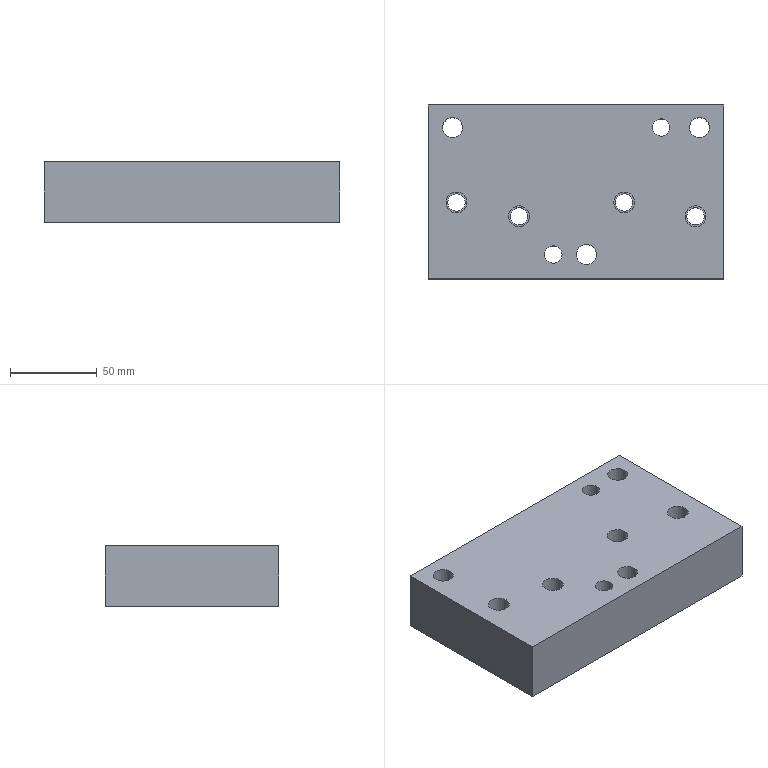Part | NX | features solid 2 | 1 solid | 45 faces | box 170 x 100 x 35 mm | volume 548006 mm3 | cylinder 24 | plane 13 | cone 8 | commonest cylinder face diameters 8.506 x8 10 x6 12 x4 11.509 x3 18.007 x3
STEP:
#1=CARTESIAN_POINT('',(1400.579,138.904,53.));
#2=VERTEX_POINT('',#1);
#3=CARTESIAN_POINT('',(1405.579,138.904,53.));
#4=DIRECTION('',(0.,0.,-1.));
#5=DIRECTION('',(-1.,0.,0.));
#6=AXIS2_PLACEMENT_3D('',#3,#4,#5);
#7=CIRCLE('',#6,5.);
#8=EDGE_CURVE('',#2,#2,#7,.T.);
#9=ORIENTED_EDGE('',*,*,#8,.F.);
#10=EDGE_LOOP('',(#9));
#11=FACE_BOUND('',#10,.T.);
#12=CARTESIAN_POINT('',(1359.579,146.904,53.));
#13=VERTEX_POINT('',#12);
#14=CARTESIAN_POINT('',(1364.579,146.904,53.));
#15=DIRECTION('',(0.,0.,-1.));
#16=DIRECTION('',(-1.,0.,0.));
#17=AXIS2_PLACEMENT_3D('',#14,#15,#16);
#18=CIRCLE('',#17,5.);
#19=EDGE_CURVE('',#13,#13,#18,.T.);
#20=ORIENTED_EDGE('',*,*,#19,.F.);
#21=EDGE_LOOP('',(#20));
#22=FACE_BOUND('',#21,.T.);
#23=CARTESIAN_POINT('',(1299.079,138.904,53.));
#24=VERTEX_POINT('',#23);
#25=CARTESIAN_POINT('',(1304.079,138.904,53.));
#26=DIRECTION('',(0.,0.,-1.));
#27=DIRECTION('',(-1.,0.,0.));
#28=AXIS2_PLACEMENT_3D('',#25,#26,#27);
#29=CIRCLE('',#28,5.);
#30=EDGE_CURVE('',#24,#24,#29,.T.);
#31=ORIENTED_EDGE('',*,*,#30,.F.);
#32=EDGE_LOOP('',(#31));
#33=FACE_BOUND('',#32,.T.);
#34=CARTESIAN_POINT('',(1263.079,146.904,53.));
#35=VERTEX_POINT('',#34);
#36=CARTESIAN_POINT('',(1268.079,146.904,53.));
#37=DIRECTION('',(0.,0.,-1.));
#38=DIRECTION('',(-1.,0.,0.));
#39=AXIS2_PLACEMENT_3D('',#36,#37,#38);
#40=CIRCLE('',#39,5.);
#41=EDGE_CURVE('',#35,#35,#40,.T.);
#42=ORIENTED_EDGE('',*,*,#41,.F.);
#43=EDGE_LOOP('',(#42));
#44=FACE_BOUND('',#43,.T.);
#45=CARTESIAN_POINT('',(1360.326,122.904,53.));
#46=VERTEX_POINT('',#45);
#47=CARTESIAN_POINT('',(1364.579,122.904,53.));
#48=DIRECTION('',(0.,0.,-1.));
#49=DIRECTION('',(-1.,0.,0.));
#50=AXIS2_PLACEMENT_3D('',#47,#48,#49);
#51=CIRCLE('',#50,4.253);
#52=EDGE_CURVE('',#46,#46,#51,.T.);
#53=ORIENTED_EDGE('',*,*,#52,.F.);
#54=EDGE_LOOP('',(#53));
#55=FACE_BOUND('',#54,.T.);
#56=CARTESIAN_POINT('',(1263.826,122.904,53.));
#57=VERTEX_POINT('',#56);
#58=CARTESIAN_POINT('',(1268.079,122.904,53.));
#59=DIRECTION('',(0.,0.,-1.));
#60=DIRECTION('',(-1.,0.,0.));
#61=AXIS2_PLACEMENT_3D('',#58,#59,#60);
#62=CIRCLE('',#61,4.253);
#63=EDGE_CURVE('',#57,#57,#62,.T.);
#64=ORIENTED_EDGE('',*,*,#63,.F.);
#65=EDGE_LOOP('',(#64));
#66=FACE_BOUND('',#65,.T.);
#67=CARTESIAN_POINT('',(1299.826,118.904,53.));
#68=VERTEX_POINT('',#67);
#69=CARTESIAN_POINT('',(1304.079,118.904,53.));
#70=DIRECTION('',(0.,0.,-1.));
#71=DIRECTION('',(-1.,0.,0.));
#72=AXIS2_PLACEMENT_3D('',#69,#70,#71);
#73=CIRCLE('',#72,4.253);
#74=EDGE_CURVE('',#68,#68,#73,.T.);
#75=ORIENTED_EDGE('',*,*,#74,.F.);
#76=EDGE_LOOP('',(#75));
#77=FACE_BOUND('',#76,.T.);
#78=CARTESIAN_POINT('',(1299.826,164.904,53.));
#79=VERTEX_POINT('',#78);
#80=CARTESIAN_POINT('',(1304.079,164.904,53.));
#81=DIRECTION('',(0.,0.,-1.));
#82=DIRECTION('',(-1.,0.,0.));
#83=AXIS2_PLACEMENT_3D('',#80,#81,#82);
#84=CIRCLE('',#83,4.253);
#85=EDGE_CURVE('',#79,#79,#84,.T.);
#86=ORIENTED_EDGE('',*,*,#85,.F.);
#87=EDGE_LOOP('',(#86));
#88=FACE_BOUND('',#87,.T.);
#89=CARTESIAN_POINT('',(1401.326,118.904,53.));
#90=VERTEX_POINT('',#89);
#91=CARTESIAN_POINT('',(1405.579,118.904,53.));
#92=DIRECTION('',(0.,0.,-1.));
#93=DIRECTION('',(-1.,0.,0.));
#94=AXIS2_PLACEMENT_3D('',#91,#92,#93);
#95=CIRCLE('',#94,4.253);
#96=EDGE_CURVE('',#90,#90,#95,.T.);
#97=ORIENTED_EDGE('',*,*,#96,.F.);
#98=EDGE_LOOP('',(#97));
#99=FACE_BOUND('',#98,.T.);
#100=CARTESIAN_POINT('',(1401.326,164.904,53.));
#101=VERTEX_POINT('',#100);
#102=CARTESIAN_POINT('',(1405.579,164.904,53.));
#103=DIRECTION('',(0.,0.,-1.));
#104=DIRECTION('',(-1.,0.,0.));
#105=AXIS2_PLACEMENT_3D('',#102,#103,#104);
#106=CIRCLE('',#105,4.253);
#107=EDGE_CURVE('',#101,#101,#106,.T.);
#108=ORIENTED_EDGE('',*,*,#107,.F.);
#109=EDGE_LOOP('',(#108));
#110=FACE_BOUND('',#109,.T.);
#111=CARTESIAN_POINT('',(1360.326,164.904,53.));
#112=VERTEX_POINT('',#111);
#113=CARTESIAN_POINT('',(1364.579,164.904,53.));
#114=DIRECTION('',(0.,0.,-1.));
#115=DIRECTION('',(-1.,0.,0.));
#116=AXIS2_PLACEMENT_3D('',#113,#114,#115);
#117=CIRCLE('',#116,4.253);
#118=EDGE_CURVE('',#112,#112,#117,.T.);
#119=ORIENTED_EDGE('',*,*,#118,.F.);
#120=EDGE_LOOP('',(#119));
#121=FACE_BOUND('',#120,.T.);
#122=CARTESIAN_POINT('',(1263.826,164.904,53.));
#123=VERTEX_POINT('',#122);
#124=CARTESIAN_POINT('',(1268.079,164.904,53.));
#125=DIRECTION('',(0.,0.,-1.));
#126=DIRECTION('',(-1.,0.,0.));
#127=AXIS2_PLACEMENT_3D('',#124,#125,#126);
#128=CIRCLE('',#127,4.253);
#129=EDGE_CURVE('',#123,#123,#128,.T.);
#130=ORIENTED_EDGE('',*,*,#129,.F.);
#131=EDGE_LOOP('',(#130));
#132=FACE_BOUND('',#131,.T.);
#133=CARTESIAN_POINT('',(1398.825,189.904,53.));
#134=VERTEX_POINT('',#133);
#135=CARTESIAN_POINT('',(1407.829,189.904,53.));
#136=DIRECTION('',(0.,0.,-1.));
#137=DIRECTION('',(-1.,0.,0.));
#138=AXIS2_PLACEMENT_3D('',#135,#136,#137);
#139=CIRCLE('',#138,9.004);
#140=EDGE_CURVE('',#134,#134,#139,.T.);
#141=ORIENTED_EDGE('',*,*,#140,.F.);
#142=EDGE_LOOP('',(#141));
#143=FACE_BOUND('',#142,.T.);
#144=CARTESIAN_POINT('',(1421.829,202.904,53.));
#145=VERTEX_POINT('',#144);
#146=CARTESIAN_POINT('',(1421.829,102.904,53.));
#147=VERTEX_POINT('',#146);
#148=CARTESIAN_POINT('',(1421.829,141.904,53.));
#149=DIRECTION('',(0.,-1.,0.));
#150=VECTOR('',#149,1000.);
#151=LINE('',#148,#150);
#152=EDGE_CURVE('',#145,#147,#151,.T.);
#153=ORIENTED_EDGE('',*,*,#152,.T.);
#154=CARTESIAN_POINT('',(1251.829,102.904,53.));
#155=VERTEX_POINT('',#154);
#156=CARTESIAN_POINT('',(1336.829,102.904,53.));
#157=DIRECTION('',(-1.,0.,0.));
#158=VECTOR('',#157,1000.);
#159=LINE('',#156,#158);
#160=EDGE_CURVE('',#147,#155,#159,.T.);
#161=ORIENTED_EDGE('',*,*,#160,.T.);
#162=CARTESIAN_POINT('',(1251.829,202.904,53.));
#163=VERTEX_POINT('',#162);
#164=CARTESIAN_POINT('',(1251.829,141.904,53.));
#165=DIRECTION('',(0.,1.,0.));
#166=VECTOR('',#165,1000.);
#167=LINE('',#164,#166);
#168=EDGE_CURVE('',#155,#163,#167,.T.);
#169=ORIENTED_EDGE('',*,*,#168,.T.);
#170=CARTESIAN_POINT('',(1336.829,202.904,53.));
#171=DIRECTION('',(1.,0.,0.));
#172=VECTOR('',#171,1000.);
#173=LINE('',#170,#172);
#174=EDGE_CURVE('',#163,#145,#173,.T.);
#175=ORIENTED_EDGE('',*,*,#174,.T.);
#176=EDGE_LOOP('',(#153,#161,#169,#175));
#177=FACE_BOUND('',#176,.T.);
#178=CARTESIAN_POINT('',(1380.829,189.904,53.));
#179=VERTEX_POINT('',#178);
#180=CARTESIAN_POINT('',(1385.829,189.904,53.));
#181=DIRECTION('',(0.,0.,-1.));
#182=DIRECTION('',(-1.,0.,0.));
#183=AXIS2_PLACEMENT_3D('',#180,#181,#182);
#184=CIRCLE('',#183,5.);
#185=EDGE_CURVE('',#179,#179,#184,.F.);
#186=ORIENTED_EDGE('',*,*,#185,.T.);
#187=EDGE_LOOP('',(#186));
#188=FACE_BOUND('',#187,.T.);
#189=CARTESIAN_POINT('',(1318.829,116.904,53.));
#190=VERTEX_POINT('',#189);
#191=CARTESIAN_POINT('',(1323.829,116.904,53.));
#192=DIRECTION('',(0.,0.,-1.));
#193=DIRECTION('',(-1.,0.,0.));
#194=AXIS2_PLACEMENT_3D('',#191,#192,#193);
#195=CIRCLE('',#194,5.);
#196=EDGE_CURVE('',#190,#190,#195,.F.);
#197=ORIENTED_EDGE('',*,*,#196,.T.);
#198=EDGE_LOOP('',(#197));
#199=FACE_BOUND('',#198,.T.);
#200=CARTESIAN_POINT('',(1333.825,116.904,53.));
#201=VERTEX_POINT('',#200);
#202=CARTESIAN_POINT('',(1342.829,116.904,53.));
#203=DIRECTION('',(0.,0.,-1.));
#204=DIRECTION('',(-1.,0.,0.));
#205=AXIS2_PLACEMENT_3D('',#202,#203,#204);
#206=CIRCLE('',#205,9.004);
#207=EDGE_CURVE('',#201,#201,#206,.T.);
#208=ORIENTED_EDGE('',*,*,#207,.F.);
#209=EDGE_LOOP('',(#208));
#210=FACE_BOUND('',#209,.T.);
#211=CARTESIAN_POINT('',(1256.825,189.904,53.));
#212=VERTEX_POINT('',#211);
#213=CARTESIAN_POINT('',(1265.829,189.904,53.));
#214=DIRECTION('',(0.,0.,-1.));
#215=DIRECTION('',(-1.,0.,0.));
#216=AXIS2_PLACEMENT_3D('',#213,#214,#215);
#217=CIRCLE('',#216,9.004);
#218=EDGE_CURVE('',#212,#212,#217,.T.);
#219=ORIENTED_EDGE('',*,*,#218,.F.);
#220=EDGE_LOOP('',(#219));
#221=FACE_BOUND('',#220,.T.);
#222=CARTESIAN_POINT('',(1336.829,141.904,53.));
#223=DIRECTION('',(0.,0.,-1.));
#224=DIRECTION('',(-1.,0.,0.));
#225=AXIS2_PLACEMENT_3D('',#222,#223,#224);
#226=PLANE('',#225);
#227=ADVANCED_FACE('',(#11,#22,#33,#44,#55,#66,#77,#88,#99,#110,#121,#132,#143,#177,#188,#199,#210,#221),#226,.T.);
#228=CARTESIAN_POINT('',(1421.829,202.904,88.));
#229=VERTEX_POINT('',#228);
#230=CARTESIAN_POINT('',(1251.829,202.904,88.));
#231=VERTEX_POINT('',#230);
#232=CARTESIAN_POINT('',(1336.829,202.904,88.));
#233=DIRECTION('',(-1.,0.,0.));
#234=VECTOR('',#233,1000.);
#235=LINE('',#232,#234);
#236=EDGE_CURVE('',#229,#231,#235,.T.);
#237=ORIENTED_EDGE('',*,*,#236,.F.);
#238=CARTESIAN_POINT('',(1421.829,202.904,50.));
#239=DIRECTION('',(0.,0.,1.));
#240=VECTOR('',#239,1000.);
#241=LINE('',#238,#240);
#242=EDGE_CURVE('',#145,#229,#241,.T.);
#243=ORIENTED_EDGE('',*,*,#242,.F.);
#244=ORIENTED_EDGE('',*,*,#174,.F.);
#245=CARTESIAN_POINT('',(1251.829,202.904,50.));
#246=DIRECTION('',(0.,0.,1.));
#247=VECTOR('',#246,1000.);
#248=LINE('',#245,#247);
#249=EDGE_CURVE('',#163,#231,#248,.T.);
#250=ORIENTED_EDGE('',*,*,#249,.T.);
#251=EDGE_LOOP('',(#237,#243,#244,#250));
#252=FACE_BOUND('',#251,.T.);
#253=CARTESIAN_POINT('',(1336.829,202.904,50.));
#254=DIRECTION('',(0.,1.,0.));
#255=DIRECTION('',(0.,0.,-1.));
#256=AXIS2_PLACEMENT_3D('',#253,#254,#255);
#257=PLANE('',#256);
#258=ADVANCED_FACE('',(#252),#257,.T.);
#259=CARTESIAN_POINT('',(1251.829,102.904,88.));
#260=VERTEX_POINT('',#259);
#261=CARTESIAN_POINT('',(1251.829,141.904,88.));
#262=DIRECTION('',(0.,-1.,0.));
#263=VECTOR('',#262,1000.);
#264=LINE('',#261,#263);
#265=EDGE_CURVE('',#231,#260,#264,.T.);
#266=ORIENTED_EDGE('',*,*,#265,.F.);
#267=ORIENTED_EDGE('',*,*,#249,.F.);
#268=ORIENTED_EDGE('',*,*,#168,.F.);
#269=CARTESIAN_POINT('',(1251.829,102.904,50.));
#270=DIRECTION('',(0.,0.,1.));
#271=VECTOR('',#270,1000.);
#272=LINE('',#269,#271);
#273=EDGE_CURVE('',#155,#260,#272,.T.);
#274=ORIENTED_EDGE('',*,*,#273,.T.);
#275=EDGE_LOOP('',(#266,#267,#268,#274));
#276=FACE_BOUND('',#275,.T.);
#277=CARTESIAN_POINT('',(1251.829,141.904,50.));
#278=DIRECTION('',(-1.,0.,0.));
#279=DIRECTION('',(0.,0.,1.));
#280=AXIS2_PLACEMENT_3D('',#277,#278,#279);
#281=PLANE('',#280);
#282=ADVANCED_FACE('',(#276),#281,.T.);
#283=CARTESIAN_POINT('',(1421.829,102.904,88.));
#284=VERTEX_POINT('',#283);
#285=CARTESIAN_POINT('',(1336.829,102.904,88.));
#286=DIRECTION('',(-1.,0.,0.));
#287=VECTOR('',#286,1000.);
#288=LINE('',#285,#287);
#289=EDGE_CURVE('',#284,#260,#288,.T.);
#290=ORIENTED_EDGE('',*,*,#289,.T.);
#291=ORIENTED_EDGE('',*,*,#273,.F.);
#292=ORIENTED_EDGE('',*,*,#160,.F.);
#293=CARTESIAN_POINT('',(1421.829,102.904,50.));
#294=DIRECTION('',(0.,0.,1.));
#295=VECTOR('',#294,1000.);
#296=LINE('',#293,#295);
#297=EDGE_CURVE('',#147,#284,#296,.T.);
#298=ORIENTED_EDGE('',*,*,#297,.T.);
#299=EDGE_LOOP('',(#290,#291,#292,#298));
#300=FACE_BOUND('',#299,.T.);
#301=CARTESIAN_POINT('',(1336.829,102.904,50.));
#302=DIRECTION('',(0.,-1.,0.));
#303=DIRECTION('',(0.,0.,1.));
#304=AXIS2_PLACEMENT_3D('',#301,#302,#303);
#305=PLANE('',#304);
#306=ADVANCED_FACE('',(#300),#305,.T.);
#307=CARTESIAN_POINT('',(1421.829,141.904,88.));
#308=DIRECTION('',(0.,-1.,0.));
#309=VECTOR('',#308,1000.);
#310=LINE('',#307,#309);
#311=EDGE_CURVE('',#229,#284,#310,.T.);
#312=ORIENTED_EDGE('',*,*,#311,.T.);
#313=ORIENTED_EDGE('',*,*,#297,.F.);
#314=ORIENTED_EDGE('',*,*,#152,.F.);
#315=ORIENTED_EDGE('',*,*,#242,.T.);
#316=EDGE_LOOP('',(#312,#313,#314,#315));
#317=FACE_BOUND('',#316,.T.);
#318=CARTESIAN_POINT('',(1421.829,141.904,50.));
#319=DIRECTION('',(1.,0.,0.));
#320=DIRECTION('',(0.,0.,-1.));
#321=AXIS2_PLACEMENT_3D('',#318,#319,#320);
#322=PLANE('',#321);
#323=ADVANCED_FACE('',(#317),#322,.T.);
#324=CARTESIAN_POINT('',(1399.579,138.904,88.));
#325=VERTEX_POINT('',#324);
#326=CARTESIAN_POINT('',(1405.579,138.904,88.));
#327=DIRECTION('',(0.,0.,-1.));
#328=DIRECTION('',(-1.,0.,0.));
#329=AXIS2_PLACEMENT_3D('',#326,#327,#328);
#330=CIRCLE('',#329,6.);
#331=EDGE_CURVE('',#325,#325,#330,.T.);
#332=ORIENTED_EDGE('',*,*,#331,.T.);
#333=EDGE_LOOP('',(#332));
#334=FACE_BOUND('',#333,.T.);
#335=CARTESIAN_POINT('',(1358.579,146.904,88.));
#336=VERTEX_POINT('',#335);
#337=CARTESIAN_POINT('',(1364.579,146.904,88.));
#338=DIRECTION('',(0.,0.,-1.));
#339=DIRECTION('',(-1.,0.,0.));
#340=AXIS2_PLACEMENT_3D('',#337,#338,#339);
#341=CIRCLE('',#340,6.);
#342=EDGE_CURVE('',#336,#336,#341,.T.);
#343=ORIENTED_EDGE('',*,*,#342,.T.);
#344=EDGE_LOOP('',(#343));
#345=FACE_BOUND('',#344,.T.);
#346=CARTESIAN_POINT('',(1298.079,138.904,88.));
#347=VERTEX_POINT('',#346);
#348=CARTESIAN_POINT('',(1304.079,138.904,88.));
#349=DIRECTION('',(0.,0.,-1.));
#350=DIRECTION('',(-1.,0.,0.));
#351=AXIS2_PLACEMENT_3D('',#348,#349,#350);
#352=CIRCLE('',#351,6.);
#353=EDGE_CURVE('',#347,#347,#352,.T.);
#354=ORIENTED_EDGE('',*,*,#353,.T.);
#355=EDGE_LOOP('',(#354));
#356=FACE_BOUND('',#355,.T.);
#357=CARTESIAN_POINT('',(1262.079,146.904,88.));
#358=VERTEX_POINT('',#357);
#359=CARTESIAN_POINT('',(1268.079,146.904,88.));
#360=DIRECTION('',(0.,0.,-1.));
#361=DIRECTION('',(-1.,0.,0.));
#362=AXIS2_PLACEMENT_3D('',#359,#360,#361);
#363=CIRCLE('',#362,6.);
#364=EDGE_CURVE('',#358,#358,#363,.T.);
#365=ORIENTED_EDGE('',*,*,#364,.T.);
#366=EDGE_LOOP('',(#365));
#367=FACE_BOUND('',#366,.T.);
#368=CARTESIAN_POINT('',(1260.074,189.904,88.));
#369=VERTEX_POINT('',#368);
#370=CARTESIAN_POINT('',(1265.829,189.904,88.));
#371=DIRECTION('',(0.,0.,1.));
#372=DIRECTION('',(-1.,0.,0.));
#373=AXIS2_PLACEMENT_3D('',#370,#371,#372);
#374=CIRCLE('',#373,5.755);
#375=EDGE_CURVE('',#369,#369,#374,.T.);
#376=ORIENTED_EDGE('',*,*,#375,.F.);
#377=EDGE_LOOP('',(#376));
#378=FACE_BOUND('',#377,.T.);
#379=CARTESIAN_POINT('',(1318.829,116.904,88.));
#380=VERTEX_POINT('',#379);
#381=CARTESIAN_POINT('',(1323.829,116.904,88.));
#382=DIRECTION('',(0.,0.,1.));
#383=DIRECTION('',(-1.,0.,0.));
#384=AXIS2_PLACEMENT_3D('',#381,#382,#383);
#385=CIRCLE('',#384,5.);
#386=EDGE_CURVE('',#380,#380,#385,.T.);
#387=ORIENTED_EDGE('',*,*,#386,.F.);
#388=EDGE_LOOP('',(#387));
#389=FACE_BOUND('',#388,.T.);
#390=CARTESIAN_POINT('',(1380.829,189.904,88.));
#391=VERTEX_POINT('',#390);
#392=CARTESIAN_POINT('',(1385.829,189.904,88.));
#393=DIRECTION('',(0.,0.,1.));
#394=DIRECTION('',(-1.,0.,0.));
#395=AXIS2_PLACEMENT_3D('',#392,#393,#394);
#396=CIRCLE('',#395,5.);
#397=EDGE_CURVE('',#391,#391,#396,.T.);
#398=ORIENTED_EDGE('',*,*,#397,.F.);
#399=EDGE_LOOP('',(#398));
#400=FACE_BOUND('',#399,.T.);
#401=CARTESIAN_POINT('',(1402.074,189.904,88.));
#402=VERTEX_POINT('',#401);
#403=CARTESIAN_POINT('',(1407.829,189.904,88.));
#404=DIRECTION('',(0.,0.,1.));
#405=DIRECTION('',(-1.,0.,0.));
#406=AXIS2_PLACEMENT_3D('',#403,#404,#405);
#407=CIRCLE('',#406,5.755);
#408=EDGE_CURVE('',#402,#402,#407,.T.);
#409=ORIENTED_EDGE('',*,*,#408,.F.);
#410=EDGE_LOOP('',(#409));
#411=FACE_BOUND('',#410,.T.);
#412=CARTESIAN_POINT('',(1337.074,116.904,88.));
#413=VERTEX_POINT('',#412);
#414=CARTESIAN_POINT('',(1342.829,116.904,88.));
#415=DIRECTION('',(0.,0.,1.));
#416=DIRECTION('',(-1.,0.,0.));
#417=AXIS2_PLACEMENT_3D('',#414,#415,#416);
#418=CIRCLE('',#417,5.755);
#419=EDGE_CURVE('',#413,#413,#418,.T.);
#420=ORIENTED_EDGE('',*,*,#419,.F.);
#421=EDGE_LOOP('',(#420));
#422=FACE_BOUND('',#421,.T.);
#423=ORIENTED_EDGE('',*,*,#236,.T.);
#424=ORIENTED_EDGE('',*,*,#265,.T.);
#425=ORIENTED_EDGE('',*,*,#289,.F.);
#426=ORIENTED_EDGE('',*,*,#311,.F.);
#427=EDGE_LOOP('',(#423,#424,#425,#426));
#428=FACE_BOUND('',#427,.T.);
#429=CARTESIAN_POINT('',(1336.829,141.904,88.));
#430=DIRECTION('',(0.,0.,-1.));
#431=DIRECTION('',(-1.,0.,0.));
#432=AXIS2_PLACEMENT_3D('',#429,#430,#431);
#433=PLANE('',#432);
#434=ADVANCED_FACE('',(#334,#345,#356,#367,#378,#389,#400,#411,#422,#428),#433,.F.);
#435=CARTESIAN_POINT('',(1348.583,116.904,63.));
#436=VERTEX_POINT('',#435);
#437=CARTESIAN_POINT('',(1342.829,116.904,63.));
#438=DIRECTION('',(0.,0.,-1.));
#439=DIRECTION('',(1.,0.,0.));
#440=AXIS2_PLACEMENT_3D('',#437,#438,#439);
#441=CIRCLE('',#440,5.755);
#442=EDGE_CURVE('',#436,#436,#441,.T.);
#443=ORIENTED_EDGE('',*,*,#442,.T.);
#444=EDGE_LOOP('',(#443));
#445=FACE_BOUND('',#444,.T.);
#446=ORIENTED_EDGE('',*,*,#419,.T.);
#447=EDGE_LOOP('',(#446));
#448=FACE_BOUND('',#447,.T.);
#449=CARTESIAN_POINT('',(1342.829,116.904,45.));
#450=DIRECTION('',(0.,0.,1.));
#451=DIRECTION('',(1.,0.,0.));
#452=AXIS2_PLACEMENT_3D('',#449,#450,#451);
#453=CYLINDRICAL_SURFACE('',#452,5.755);
#454=ADVANCED_FACE('',(#445,#448),#453,.F.);
#455=ORIENTED_EDGE('',*,*,#442,.F.);
#456=EDGE_LOOP('',(#455));
#457=FACE_BOUND('',#456,.T.);
#458=CARTESIAN_POINT('',(1351.832,116.904,63.));
#459=VERTEX_POINT('',#458);
#460=CARTESIAN_POINT('',(1342.829,116.904,63.));
#461=DIRECTION('',(0.,0.,1.));
#462=DIRECTION('',(1.,0.,0.));
#463=AXIS2_PLACEMENT_3D('',#460,#461,#462);
#464=CIRCLE('',#463,9.004);
#465=EDGE_CURVE('',#459,#459,#464,.F.);
#466=ORIENTED_EDGE('',*,*,#465,.T.);
#467=EDGE_LOOP('',(#466));
#468=FACE_BOUND('',#467,.T.);
#469=CARTESIAN_POINT('',(1342.829,116.904,63.));
#470=DIRECTION('',(0.,0.,1.));
#471=DIRECTION('',(1.,0.,0.));
#472=AXIS2_PLACEMENT_3D('',#469,#470,#471);
#473=PLANE('',#472);
#474=ADVANCED_FACE('',(#457,#468),#473,.F.);
#475=ORIENTED_EDGE('',*,*,#465,.F.);
#476=EDGE_LOOP('',(#475));
#477=FACE_BOUND('',#476,.T.);
#478=ORIENTED_EDGE('',*,*,#207,.T.);
#479=EDGE_LOOP('',(#478));
#480=FACE_BOUND('',#479,.T.);
#481=CARTESIAN_POINT('',(1342.829,116.904,50.));
#482=DIRECTION('',(0.,0.,1.));
#483=DIRECTION('',(1.,0.,0.));
#484=AXIS2_PLACEMENT_3D('',#481,#482,#483);
#485=CYLINDRICAL_SURFACE('',#484,9.004);
#486=ADVANCED_FACE('',(#477,#480),#485,.F.);
#487=CARTESIAN_POINT('',(1413.583,189.904,63.));
#488=VERTEX_POINT('',#487);
#489=CARTESIAN_POINT('',(1407.829,189.904,63.));
#490=DIRECTION('',(0.,0.,-1.));
#491=DIRECTION('',(1.,0.,0.));
#492=AXIS2_PLACEMENT_3D('',#489,#490,#491);
#493=CIRCLE('',#492,5.755);
#494=EDGE_CURVE('',#488,#488,#493,.T.);
#495=ORIENTED_EDGE('',*,*,#494,.T.);
#496=EDGE_LOOP('',(#495));
#497=FACE_BOUND('',#496,.T.);
#498=ORIENTED_EDGE('',*,*,#408,.T.);
#499=EDGE_LOOP('',(#498));
#500=FACE_BOUND('',#499,.T.);
#501=CARTESIAN_POINT('',(1407.829,189.904,45.));
#502=DIRECTION('',(0.,0.,1.));
#503=DIRECTION('',(1.,0.,0.));
#504=AXIS2_PLACEMENT_3D('',#501,#502,#503);
#505=CYLINDRICAL_SURFACE('',#504,5.755);
#506=ADVANCED_FACE('',(#497,#500),#505,.F.);
#507=ORIENTED_EDGE('',*,*,#494,.F.);
#508=EDGE_LOOP('',(#507));
#509=FACE_BOUND('',#508,.T.);
#510=CARTESIAN_POINT('',(1416.832,189.904,63.));
#511=VERTEX_POINT('',#510);
#512=CARTESIAN_POINT('',(1407.829,189.904,63.));
#513=DIRECTION('',(0.,0.,1.));
#514=DIRECTION('',(1.,0.,0.));
#515=AXIS2_PLACEMENT_3D('',#512,#513,#514);
#516=CIRCLE('',#515,9.004);
#517=EDGE_CURVE('',#511,#511,#516,.F.);
#518=ORIENTED_EDGE('',*,*,#517,.T.);
#519=EDGE_LOOP('',(#518));
#520=FACE_BOUND('',#519,.T.);
#521=CARTESIAN_POINT('',(1407.829,189.904,63.));
#522=DIRECTION('',(0.,0.,1.));
#523=DIRECTION('',(1.,0.,0.));
#524=AXIS2_PLACEMENT_3D('',#521,#522,#523);
#525=PLANE('',#524);
#526=ADVANCED_FACE('',(#509,#520),#525,.F.);
#527=ORIENTED_EDGE('',*,*,#517,.F.);
#528=EDGE_LOOP('',(#527));
#529=FACE_BOUND('',#528,.T.);
#530=ORIENTED_EDGE('',*,*,#140,.T.);
#531=EDGE_LOOP('',(#530));
#532=FACE_BOUND('',#531,.T.);
#533=CARTESIAN_POINT('',(1407.829,189.904,50.));
#534=DIRECTION('',(0.,0.,1.));
#535=DIRECTION('',(1.,0.,0.));
#536=AXIS2_PLACEMENT_3D('',#533,#534,#535);
#537=CYLINDRICAL_SURFACE('',#536,9.004);
#538=ADVANCED_FACE('',(#529,#532),#537,.F.);
#539=ORIENTED_EDGE('',*,*,#185,.F.);
#540=EDGE_LOOP('',(#539));
#541=FACE_BOUND('',#540,.T.);
#542=ORIENTED_EDGE('',*,*,#397,.T.);
#543=EDGE_LOOP('',(#542));
#544=FACE_BOUND('',#543,.T.);
#545=CARTESIAN_POINT('',(1385.829,189.904,45.));
#546=DIRECTION('',(0.,0.,1.));
#547=DIRECTION('',(1.,0.,0.));
#548=AXIS2_PLACEMENT_3D('',#545,#546,#547);
#549=CYLINDRICAL_SURFACE('',#548,5.);
#550=ADVANCED_FACE('',(#541,#544),#549,.F.);
#551=ORIENTED_EDGE('',*,*,#196,.F.);
#552=EDGE_LOOP('',(#551));
#553=FACE_BOUND('',#552,.T.);
#554=ORIENTED_EDGE('',*,*,#386,.T.);
#555=EDGE_LOOP('',(#554));
#556=FACE_BOUND('',#555,.T.);
#557=CARTESIAN_POINT('',(1323.829,116.904,45.));
#558=DIRECTION('',(0.,0.,1.));
#559=DIRECTION('',(1.,0.,0.));
#560=AXIS2_PLACEMENT_3D('',#557,#558,#559);
#561=CYLINDRICAL_SURFACE('',#560,5.);
#562=ADVANCED_FACE('',(#553,#556),#561,.F.);
#563=CARTESIAN_POINT('',(1271.583,189.904,63.));
#564=VERTEX_POINT('',#563);
#565=CARTESIAN_POINT('',(1265.829,189.904,63.));
#566=DIRECTION('',(0.,0.,-1.));
#567=DIRECTION('',(1.,0.,0.));
#568=AXIS2_PLACEMENT_3D('',#565,#566,#567);
#569=CIRCLE('',#568,5.755);
#570=EDGE_CURVE('',#564,#564,#569,.T.);
#571=ORIENTED_EDGE('',*,*,#570,.T.);
#572=EDGE_LOOP('',(#571));
#573=FACE_BOUND('',#572,.T.);
#574=ORIENTED_EDGE('',*,*,#375,.T.);
#575=EDGE_LOOP('',(#574));
#576=FACE_BOUND('',#575,.T.);
#577=CARTESIAN_POINT('',(1265.829,189.904,45.));
#578=DIRECTION('',(0.,0.,1.));
#579=DIRECTION('',(1.,0.,0.));
#580=AXIS2_PLACEMENT_3D('',#577,#578,#579);
#581=CYLINDRICAL_SURFACE('',#580,5.755);
#582=ADVANCED_FACE('',(#573,#576),#581,.F.);
#583=ORIENTED_EDGE('',*,*,#570,.F.);
#584=EDGE_LOOP('',(#583));
#585=FACE_BOUND('',#584,.T.);
#586=CARTESIAN_POINT('',(1274.832,189.904,63.));
#587=VERTEX_POINT('',#586);
#588=CARTESIAN_POINT('',(1265.829,189.904,63.));
#589=DIRECTION('',(0.,0.,1.));
#590=DIRECTION('',(1.,0.,0.));
#591=AXIS2_PLACEMENT_3D('',#588,#589,#590);
#592=CIRCLE('',#591,9.004);
#593=EDGE_CURVE('',#587,#587,#592,.F.);
#594=ORIENTED_EDGE('',*,*,#593,.T.);
#595=EDGE_LOOP('',(#594));
#596=FACE_BOUND('',#595,.T.);
#597=CARTESIAN_POINT('',(1265.829,189.904,63.));
#598=DIRECTION('',(0.,0.,1.));
#599=DIRECTION('',(1.,0.,0.));
#600=AXIS2_PLACEMENT_3D('',#597,#598,#599);
#601=PLANE('',#600);
#602=ADVANCED_FACE('',(#585,#596),#601,.F.);
#603=ORIENTED_EDGE('',*,*,#593,.F.);
#604=EDGE_LOOP('',(#603));
#605=FACE_BOUND('',#604,.T.);
#606=ORIENTED_EDGE('',*,*,#218,.T.);
#607=EDGE_LOOP('',(#606));
#608=FACE_BOUND('',#607,.T.);
#609=CARTESIAN_POINT('',(1265.829,189.904,50.));
#610=DIRECTION('',(0.,0.,1.));
#611=DIRECTION('',(1.,0.,0.));
#612=AXIS2_PLACEMENT_3D('',#609,#610,#611);
#613=CYLINDRICAL_SURFACE('',#612,9.004);
#614=ADVANCED_FACE('',(#605,#608),#613,.F.);
#615=ORIENTED_EDGE('',*,*,#129,.T.);
#616=EDGE_LOOP('',(#615));
#617=FACE_BOUND('',#616,.T.);
#618=CARTESIAN_POINT('',(1263.826,164.904,80.753));
#619=VERTEX_POINT('',#618);
#620=CARTESIAN_POINT('',(1268.079,164.904,80.753));
#621=DIRECTION('',(0.,0.,-1.));
#622=DIRECTION('',(-1.,0.,0.));
#623=AXIS2_PLACEMENT_3D('',#620,#621,#622);
#624=CIRCLE('',#623,4.253);
#625=EDGE_CURVE('',#619,#619,#624,.T.);
#626=ORIENTED_EDGE('',*,*,#625,.F.);
#627=EDGE_LOOP('',(#626));
#628=FACE_BOUND('',#627,.T.);
#629=CARTESIAN_POINT('',(1268.079,164.904,50.));
#630=DIRECTION('',(0.,0.,1.));
#631=DIRECTION('',(1.,0.,0.));
#632=AXIS2_PLACEMENT_3D('',#629,#630,#631);
#633=CYLINDRICAL_SURFACE('',#632,4.253);
#634=ADVANCED_FACE('',(#617,#628),#633,.F.);
#635=CARTESIAN_POINT('',(1268.079,164.904,85.006));
#636=VERTEX_POINT('',#635);
#637=VERTEX_LOOP('',#636);
#638=FACE_BOUND('',#637,.T.);
#639=ORIENTED_EDGE('',*,*,#625,.T.);
#640=EDGE_LOOP('',(#639));
#641=FACE_BOUND('',#640,.T.);
#642=CARTESIAN_POINT('',(1268.079,164.904,80.753));
#643=DIRECTION('',(0.,0.,-1.));
#644=DIRECTION('',(1.,0.,0.));
#645=AXIS2_PLACEMENT_3D('',#642,#643,#644);
#646=CONICAL_SURFACE('',#645,4.253,0.7854);
#647=ADVANCED_FACE('',(#638,#641),#646,.F.);
#648=ORIENTED_EDGE('',*,*,#118,.T.);
#649=EDGE_LOOP('',(#648));
#650=FACE_BOUND('',#649,.T.);
#651=CARTESIAN_POINT('',(1360.326,164.904,80.753));
#652=VERTEX_POINT('',#651);
#653=CARTESIAN_POINT('',(1364.579,164.904,80.753));
#654=DIRECTION('',(0.,0.,-1.));
#655=DIRECTION('',(-1.,0.,0.));
#656=AXIS2_PLACEMENT_3D('',#653,#654,#655);
#657=CIRCLE('',#656,4.253);
#658=EDGE_CURVE('',#652,#652,#657,.T.);
#659=ORIENTED_EDGE('',*,*,#658,.F.);
#660=EDGE_LOOP('',(#659));
#661=FACE_BOUND('',#660,.T.);
#662=CARTESIAN_POINT('',(1364.579,164.904,50.));
#663=DIRECTION('',(0.,0.,1.));
#664=DIRECTION('',(1.,0.,0.));
#665=AXIS2_PLACEMENT_3D('',#662,#663,#664);
#666=CYLINDRICAL_SURFACE('',#665,4.253);
#667=ADVANCED_FACE('',(#650,#661),#666,.F.);
#668=CARTESIAN_POINT('',(1364.579,164.904,85.006));
#669=VERTEX_POINT('',#668);
#670=VERTEX_LOOP('',#669);
#671=FACE_BOUND('',#670,.T.);
#672=ORIENTED_EDGE('',*,*,#658,.T.);
#673=EDGE_LOOP('',(#672));
#674=FACE_BOUND('',#673,.T.);
#675=CARTESIAN_POINT('',(1364.579,164.904,80.753));
#676=DIRECTION('',(0.,0.,-1.));
#677=DIRECTION('',(1.,0.,0.));
#678=AXIS2_PLACEMENT_3D('',#675,#676,#677);
#679=CONICAL_SURFACE('',#678,4.253,0.7854);
#680=ADVANCED_FACE('',(#671,#674),#679,.F.);
#681=ORIENTED_EDGE('',*,*,#107,.T.);
#682=EDGE_LOOP('',(#681));
#683=FACE_BOUND('',#682,.T.);
#684=CARTESIAN_POINT('',(1401.326,164.904,80.753));
#685=VERTEX_POINT('',#684);
#686=CARTESIAN_POINT('',(1405.579,164.904,80.753));
#687=DIRECTION('',(0.,0.,-1.));
#688=DIRECTION('',(-1.,0.,0.));
#689=AXIS2_PLACEMENT_3D('',#686,#687,#688);
#690=CIRCLE('',#689,4.253);
#691=EDGE_CURVE('',#685,#685,#690,.T.);
#692=ORIENTED_EDGE('',*,*,#691,.F.);
#693=EDGE_LOOP('',(#692));
#694=FACE_BOUND('',#693,.T.);
#695=CARTESIAN_POINT('',(1405.579,164.904,50.));
#696=DIRECTION('',(0.,0.,1.));
#697=DIRECTION('',(1.,0.,0.));
#698=AXIS2_PLACEMENT_3D('',#695,#696,#697);
#699=CYLINDRICAL_SURFACE('',#698,4.253);
#700=ADVANCED_FACE('',(#683,#694),#699,.F.);
#701=CARTESIAN_POINT('',(1405.579,164.904,85.006));
#702=VERTEX_POINT('',#701);
#703=VERTEX_LOOP('',#702);
#704=FACE_BOUND('',#703,.T.);
#705=ORIENTED_EDGE('',*,*,#691,.T.);
#706=EDGE_LOOP('',(#705));
#707=FACE_BOUND('',#706,.T.);
#708=CARTESIAN_POINT('',(1405.579,164.904,80.753));
#709=DIRECTION('',(0.,0.,-1.));
#710=DIRECTION('',(1.,0.,0.));
#711=AXIS2_PLACEMENT_3D('',#708,#709,#710);
#712=CONICAL_SURFACE('',#711,4.253,0.7854);
#713=ADVANCED_FACE('',(#704,#707),#712,.F.);
#714=ORIENTED_EDGE('',*,*,#96,.T.);
#715=EDGE_LOOP('',(#714));
#716=FACE_BOUND('',#715,.T.);
#717=CARTESIAN_POINT('',(1401.326,118.904,80.753));
#718=VERTEX_POINT('',#717);
#719=CARTESIAN_POINT('',(1405.579,118.904,80.753));
#720=DIRECTION('',(0.,0.,-1.));
#721=DIRECTION('',(-1.,0.,0.));
#722=AXIS2_PLACEMENT_3D('',#719,#720,#721);
#723=CIRCLE('',#722,4.253);
#724=EDGE_CURVE('',#718,#718,#723,.T.);
#725=ORIENTED_EDGE('',*,*,#724,.F.);
#726=EDGE_LOOP('',(#725));
#727=FACE_BOUND('',#726,.T.);
#728=CARTESIAN_POINT('',(1405.579,118.904,50.));
#729=DIRECTION('',(0.,0.,1.));
#730=DIRECTION('',(1.,0.,0.));
#731=AXIS2_PLACEMENT_3D('',#728,#729,#730);
#732=CYLINDRICAL_SURFACE('',#731,4.253);
#733=ADVANCED_FACE('',(#716,#727),#732,.F.);
#734=CARTESIAN_POINT('',(1405.579,118.904,85.006));
#735=VERTEX_POINT('',#734);
#736=VERTEX_LOOP('',#735);
#737=FACE_BOUND('',#736,.T.);
#738=ORIENTED_EDGE('',*,*,#724,.T.);
#739=EDGE_LOOP('',(#738));
#740=FACE_BOUND('',#739,.T.);
#741=CARTESIAN_POINT('',(1405.579,118.904,80.753));
#742=DIRECTION('',(0.,0.,-1.));
#743=DIRECTION('',(1.,0.,0.));
#744=AXIS2_PLACEMENT_3D('',#741,#742,#743);
#745=CONICAL_SURFACE('',#744,4.253,0.7854);
#746=ADVANCED_FACE('',(#737,#740),#745,.F.);
#747=ORIENTED_EDGE('',*,*,#85,.T.);
#748=EDGE_LOOP('',(#747));
#749=FACE_BOUND('',#748,.T.);
#750=CARTESIAN_POINT('',(1299.826,164.904,80.753));
#751=VERTEX_POINT('',#750);
#752=CARTESIAN_POINT('',(1304.079,164.904,80.753));
#753=DIRECTION('',(0.,0.,-1.));
#754=DIRECTION('',(-1.,0.,0.));
#755=AXIS2_PLACEMENT_3D('',#752,#753,#754);
#756=CIRCLE('',#755,4.253);
#757=EDGE_CURVE('',#751,#751,#756,.T.);
#758=ORIENTED_EDGE('',*,*,#757,.F.);
#759=EDGE_LOOP('',(#758));
#760=FACE_BOUND('',#759,.T.);
#761=CARTESIAN_POINT('',(1304.079,164.904,50.));
#762=DIRECTION('',(0.,0.,1.));
#763=DIRECTION('',(1.,0.,0.));
#764=AXIS2_PLACEMENT_3D('',#761,#762,#763);
#765=CYLINDRICAL_SURFACE('',#764,4.253);
#766=ADVANCED_FACE('',(#749,#760),#765,.F.);
#767=CARTESIAN_POINT('',(1304.079,164.904,85.006));
#768=VERTEX_POINT('',#767);
#769=VERTEX_LOOP('',#768);
#770=FACE_BOUND('',#769,.T.);
#771=ORIENTED_EDGE('',*,*,#757,.T.);
#772=EDGE_LOOP('',(#771));
#773=FACE_BOUND('',#772,.T.);
#774=CARTESIAN_POINT('',(1304.079,164.904,80.753));
#775=DIRECTION('',(0.,0.,-1.));
#776=DIRECTION('',(1.,0.,0.));
#777=AXIS2_PLACEMENT_3D('',#774,#775,#776);
#778=CONICAL_SURFACE('',#777,4.253,0.7854);
#779=ADVANCED_FACE('',(#770,#773),#778,.F.);
#780=ORIENTED_EDGE('',*,*,#74,.T.);
#781=EDGE_LOOP('',(#780));
#782=FACE_BOUND('',#781,.T.);
#783=CARTESIAN_POINT('',(1299.826,118.904,80.753));
#784=VERTEX_POINT('',#783);
#785=CARTESIAN_POINT('',(1304.079,118.904,80.753));
#786=DIRECTION('',(0.,0.,-1.));
#787=DIRECTION('',(-1.,0.,0.));
#788=AXIS2_PLACEMENT_3D('',#785,#786,#787);
#789=CIRCLE('',#788,4.253);
#790=EDGE_CURVE('',#784,#784,#789,.T.);
#791=ORIENTED_EDGE('',*,*,#790,.F.);
#792=EDGE_LOOP('',(#791));
#793=FACE_BOUND('',#792,.T.);
#794=CARTESIAN_POINT('',(1304.079,118.904,50.));
#795=DIRECTION('',(0.,0.,1.));
#796=DIRECTION('',(1.,0.,0.));
#797=AXIS2_PLACEMENT_3D('',#794,#795,#796);
#798=CYLINDRICAL_SURFACE('',#797,4.253);
#799=ADVANCED_FACE('',(#782,#793),#798,.F.);
#800=CARTESIAN_POINT('',(1304.079,118.904,85.006));
#801=VERTEX_POINT('',#800);
#802=VERTEX_LOOP('',#801);
#803=FACE_BOUND('',#802,.T.);
#804=ORIENTED_EDGE('',*,*,#790,.T.);
#805=EDGE_LOOP('',(#804));
#806=FACE_BOUND('',#805,.T.);
#807=CARTESIAN_POINT('',(1304.079,118.904,80.753));
#808=DIRECTION('',(0.,0.,-1.));
#809=DIRECTION('',(1.,0.,0.));
#810=AXIS2_PLACEMENT_3D('',#807,#808,#809);
#811=CONICAL_SURFACE('',#810,4.253,0.7854);
#812=ADVANCED_FACE('',(#803,#806),#811,.F.);
#813=ORIENTED_EDGE('',*,*,#63,.T.);
#814=EDGE_LOOP('',(#813));
#815=FACE_BOUND('',#814,.T.);
#816=CARTESIAN_POINT('',(1263.826,122.904,80.753));
#817=VERTEX_POINT('',#816);
#818=CARTESIAN_POINT('',(1268.079,122.904,80.753));
#819=DIRECTION('',(0.,0.,-1.));
#820=DIRECTION('',(-1.,0.,0.));
#821=AXIS2_PLACEMENT_3D('',#818,#819,#820);
#822=CIRCLE('',#821,4.253);
#823=EDGE_CURVE('',#817,#817,#822,.T.);
#824=ORIENTED_EDGE('',*,*,#823,.F.);
#825=EDGE_LOOP('',(#824));
#826=FACE_BOUND('',#825,.T.);
#827=CARTESIAN_POINT('',(1268.079,122.904,50.));
#828=DIRECTION('',(0.,0.,1.));
#829=DIRECTION('',(1.,0.,0.));
#830=AXIS2_PLACEMENT_3D('',#827,#828,#829);
#831=CYLINDRICAL_SURFACE('',#830,4.253);
#832=ADVANCED_FACE('',(#815,#826),#831,.F.);
#833=CARTESIAN_POINT('',(1268.079,122.904,85.006));
#834=VERTEX_POINT('',#833);
#835=VERTEX_LOOP('',#834);
#836=FACE_BOUND('',#835,.T.);
#837=ORIENTED_EDGE('',*,*,#823,.T.);
#838=EDGE_LOOP('',(#837));
#839=FACE_BOUND('',#838,.T.);
#840=CARTESIAN_POINT('',(1268.079,122.904,80.753));
#841=DIRECTION('',(0.,0.,-1.));
#842=DIRECTION('',(1.,0.,0.));
#843=AXIS2_PLACEMENT_3D('',#840,#841,#842);
#844=CONICAL_SURFACE('',#843,4.253,0.7854);
#845=ADVANCED_FACE('',(#836,#839),#844,.F.);
#846=ORIENTED_EDGE('',*,*,#52,.T.);
#847=EDGE_LOOP('',(#846));
#848=FACE_BOUND('',#847,.T.);
#849=CARTESIAN_POINT('',(1360.326,122.904,80.753));
#850=VERTEX_POINT('',#849);
#851=CARTESIAN_POINT('',(1364.579,122.904,80.753));
#852=DIRECTION('',(0.,0.,-1.));
#853=DIRECTION('',(-1.,0.,0.));
#854=AXIS2_PLACEMENT_3D('',#851,#852,#853);
#855=CIRCLE('',#854,4.253);
#856=EDGE_CURVE('',#850,#850,#855,.T.);
#857=ORIENTED_EDGE('',*,*,#856,.F.);
#858=EDGE_LOOP('',(#857));
#859=FACE_BOUND('',#858,.T.);
#860=CARTESIAN_POINT('',(1364.579,122.904,50.));
#861=DIRECTION('',(0.,0.,1.));
#862=DIRECTION('',(1.,0.,0.));
#863=AXIS2_PLACEMENT_3D('',#860,#861,#862);
#864=CYLINDRICAL_SURFACE('',#863,4.253);
#865=ADVANCED_FACE('',(#848,#859),#864,.F.);
#866=CARTESIAN_POINT('',(1364.579,122.904,85.006));
#867=VERTEX_POINT('',#866);
#868=VERTEX_LOOP('',#867);
#869=FACE_BOUND('',#868,.T.);
#870=ORIENTED_EDGE('',*,*,#856,.T.);
#871=EDGE_LOOP('',(#870));
#872=FACE_BOUND('',#871,.T.);
#873=CARTESIAN_POINT('',(1364.579,122.904,80.753));
#874=DIRECTION('',(0.,0.,-1.));
#875=DIRECTION('',(1.,0.,0.));
#876=AXIS2_PLACEMENT_3D('',#873,#874,#875);
#877=CONICAL_SURFACE('',#876,4.253,0.7854);
#878=ADVANCED_FACE('',(#869,#872),#877,.F.);
#879=CARTESIAN_POINT('',(1262.079,146.904,75.));
#880=VERTEX_POINT('',#879);
#881=CARTESIAN_POINT('',(1268.079,146.904,75.));
#882=DIRECTION('',(0.,0.,-1.));
#883=DIRECTION('',(-1.,0.,0.));
#884=AXIS2_PLACEMENT_3D('',#881,#882,#883);
#885=CIRCLE('',#884,6.);
#886=EDGE_CURVE('',#880,#880,#885,.T.);
#887=ORIENTED_EDGE('',*,*,#886,.T.);
#888=EDGE_LOOP('',(#887));
#889=FACE_BOUND('',#888,.T.);
#890=ORIENTED_EDGE('',*,*,#364,.F.);
#891=EDGE_LOOP('',(#890));
#892=FACE_BOUND('',#891,.T.);
#893=CARTESIAN_POINT('',(1268.079,146.904,131.));
#894=DIRECTION('',(0.,0.,-1.));
#895=DIRECTION('',(1.,0.,0.));
#896=AXIS2_PLACEMENT_3D('',#893,#894,#895);
#897=CYLINDRICAL_SURFACE('',#896,6.);
#898=ADVANCED_FACE('',(#889,#892),#897,.F.);
#899=ORIENTED_EDGE('',*,*,#41,.T.);
#900=EDGE_LOOP('',(#899));
#901=FACE_BOUND('',#900,.T.);
#902=CARTESIAN_POINT('',(1263.079,146.904,75.));
#903=VERTEX_POINT('',#902);
#904=CARTESIAN_POINT('',(1268.079,146.904,75.));
#905=DIRECTION('',(0.,0.,-1.));
#906=DIRECTION('',(-1.,0.,0.));
#907=AXIS2_PLACEMENT_3D('',#904,#905,#906);
#908=CIRCLE('',#907,5.);
#909=EDGE_CURVE('',#903,#903,#908,.T.);
#910=ORIENTED_EDGE('',*,*,#909,.F.);
#911=EDGE_LOOP('',(#910));
#912=FACE_BOUND('',#911,.T.);
#913=CARTESIAN_POINT('',(1268.079,146.904,131.));
#914=DIRECTION('',(0.,0.,-1.));
#915=DIRECTION('',(1.,0.,0.));
#916=AXIS2_PLACEMENT_3D('',#913,#914,#915);
#917=CYLINDRICAL_SURFACE('',#916,5.);
#918=ADVANCED_FACE('',(#901,#912),#917,.F.);
#919=ORIENTED_EDGE('',*,*,#909,.T.);
#920=EDGE_LOOP('',(#919));
#921=FACE_BOUND('',#920,.T.);
#922=ORIENTED_EDGE('',*,*,#886,.F.);
#923=EDGE_LOOP('',(#922));
#924=FACE_BOUND('',#923,.T.);
#925=CARTESIAN_POINT('',(1268.079,146.904,75.));
#926=DIRECTION('',(0.,0.,-1.));
#927=DIRECTION('',(-1.,0.,0.));
#928=AXIS2_PLACEMENT_3D('',#925,#926,#927);
#929=PLANE('',#928);
#930=ADVANCED_FACE('',(#921,#924),#929,.F.);
#931=CARTESIAN_POINT('',(1298.079,138.904,75.));
#932=VERTEX_POINT('',#931);
#933=CARTESIAN_POINT('',(1304.079,138.904,75.));
#934=DIRECTION('',(0.,0.,-1.));
#935=DIRECTION('',(-1.,0.,0.));
#936=AXIS2_PLACEMENT_3D('',#933,#934,#935);
#937=CIRCLE('',#936,6.);
#938=EDGE_CURVE('',#932,#932,#937,.T.);
#939=ORIENTED_EDGE('',*,*,#938,.T.);
#940=EDGE_LOOP('',(#939));
#941=FACE_BOUND('',#940,.T.);
#942=ORIENTED_EDGE('',*,*,#353,.F.);
#943=EDGE_LOOP('',(#942));
#944=FACE_BOUND('',#943,.T.);
#945=CARTESIAN_POINT('',(1304.079,138.904,131.));
#946=DIRECTION('',(0.,0.,-1.));
#947=DIRECTION('',(1.,0.,0.));
#948=AXIS2_PLACEMENT_3D('',#945,#946,#947);
#949=CYLINDRICAL_SURFACE('',#948,6.);
#950=ADVANCED_FACE('',(#941,#944),#949,.F.);
#951=ORIENTED_EDGE('',*,*,#30,.T.);
#952=EDGE_LOOP('',(#951));
#953=FACE_BOUND('',#952,.T.);
#954=CARTESIAN_POINT('',(1299.079,138.904,75.));
#955=VERTEX_POINT('',#954);
#956=CARTESIAN_POINT('',(1304.079,138.904,75.));
#957=DIRECTION('',(0.,0.,-1.));
#958=DIRECTION('',(-1.,0.,0.));
#959=AXIS2_PLACEMENT_3D('',#956,#957,#958);
#960=CIRCLE('',#959,5.);
#961=EDGE_CURVE('',#955,#955,#960,.T.);
#962=ORIENTED_EDGE('',*,*,#961,.F.);
#963=EDGE_LOOP('',(#962));
#964=FACE_BOUND('',#963,.T.);
#965=CARTESIAN_POINT('',(1304.079,138.904,131.));
#966=DIRECTION('',(0.,0.,-1.));
#967=DIRECTION('',(1.,0.,0.));
#968=AXIS2_PLACEMENT_3D('',#965,#966,#967);
#969=CYLINDRICAL_SURFACE('',#968,5.);
#970=ADVANCED_FACE('',(#953,#964),#969,.F.);
#971=ORIENTED_EDGE('',*,*,#961,.T.);
#972=EDGE_LOOP('',(#971));
#973=FACE_BOUND('',#972,.T.);
#974=ORIENTED_EDGE('',*,*,#938,.F.);
#975=EDGE_LOOP('',(#974));
#976=FACE_BOUND('',#975,.T.);
#977=CARTESIAN_POINT('',(1304.079,138.904,75.));
#978=DIRECTION('',(0.,0.,-1.));
#979=DIRECTION('',(-1.,0.,0.));
#980=AXIS2_PLACEMENT_3D('',#977,#978,#979);
#981=PLANE('',#980);
#982=ADVANCED_FACE('',(#973,#976),#981,.F.);
#983=CARTESIAN_POINT('',(1358.579,146.904,75.));
#984=VERTEX_POINT('',#983);
#985=CARTESIAN_POINT('',(1364.579,146.904,75.));
#986=DIRECTION('',(0.,0.,-1.));
#987=DIRECTION('',(-1.,0.,0.));
#988=AXIS2_PLACEMENT_3D('',#985,#986,#987);
#989=CIRCLE('',#988,6.);
#990=EDGE_CURVE('',#984,#984,#989,.T.);
#991=ORIENTED_EDGE('',*,*,#990,.T.);
#992=EDGE_LOOP('',(#991));
#993=FACE_BOUND('',#992,.T.);
#994=ORIENTED_EDGE('',*,*,#342,.F.);
#995=EDGE_LOOP('',(#994));
#996=FACE_BOUND('',#995,.T.);
#997=CARTESIAN_POINT('',(1364.579,146.904,131.));
#998=DIRECTION('',(0.,0.,-1.));
#999=DIRECTION('',(1.,0.,0.));
#1000=AXIS2_PLACEMENT_3D('',#997,#998,#999);
#1001=CYLINDRICAL_SURFACE('',#1000,6.);
#1002=ADVANCED_FACE('',(#993,#996),#1001,.F.);
#1003=ORIENTED_EDGE('',*,*,#19,.T.);
#1004=EDGE_LOOP('',(#1003));
#1005=FACE_BOUND('',#1004,.T.);
#1006=CARTESIAN_POINT('',(1359.579,146.904,75.));
#1007=VERTEX_POINT('',#1006);
#1008=CARTESIAN_POINT('',(1364.579,146.904,75.));
#1009=DIRECTION('',(0.,0.,-1.));
#1010=DIRECTION('',(-1.,0.,0.));
#1011=AXIS2_PLACEMENT_3D('',#1008,#1009,#1010);
#1012=CIRCLE('',#1011,5.);
#1013=EDGE_CURVE('',#1007,#1007,#1012,.T.);
#1014=ORIENTED_EDGE('',*,*,#1013,.F.);
#1015=EDGE_LOOP('',(#1014));
#1016=FACE_BOUND('',#1015,.T.);
#1017=CARTESIAN_POINT('',(1364.579,146.904,131.));
#1018=DIRECTION('',(0.,0.,-1.));
#1019=DIRECTION('',(1.,0.,0.));
#1020=AXIS2_PLACEMENT_3D('',#1017,#1018,#1019);
#1021=CYLINDRICAL_SURFACE('',#1020,5.);
#1022=ADVANCED_FACE('',(#1005,#1016),#1021,.F.);
#1023=ORIENTED_EDGE('',*,*,#1013,.T.);
#1024=EDGE_LOOP('',(#1023));
#1025=FACE_BOUND('',#1024,.T.);
#1026=ORIENTED_EDGE('',*,*,#990,.F.);
#1027=EDGE_LOOP('',(#1026));
#1028=FACE_BOUND('',#1027,.T.);
#1029=CARTESIAN_POINT('',(1364.579,146.904,75.));
#1030=DIRECTION('',(0.,0.,-1.));
#1031=DIRECTION('',(-1.,0.,0.));
#1032=AXIS2_PLACEMENT_3D('',#1029,#1030,#1031);
#1033=PLANE('',#1032);
#1034=ADVANCED_FACE('',(#1025,#1028),#1033,.F.);
#1035=CARTESIAN_POINT('',(1399.579,138.904,75.));
#1036=VERTEX_POINT('',#1035);
#1037=CARTESIAN_POINT('',(1405.579,138.904,75.));
#1038=DIRECTION('',(0.,0.,-1.));
#1039=DIRECTION('',(-1.,0.,0.));
#1040=AXIS2_PLACEMENT_3D('',#1037,#1038,#1039);
#1041=CIRCLE('',#1040,6.);
#1042=EDGE_CURVE('',#1036,#1036,#1041,.T.);
#1043=ORIENTED_EDGE('',*,*,#1042,.T.);
#1044=EDGE_LOOP('',(#1043));
#1045=FACE_BOUND('',#1044,.T.);
#1046=ORIENTED_EDGE('',*,*,#331,.F.);
#1047=EDGE_LOOP('',(#1046));
#1048=FACE_BOUND('',#1047,.T.);
#1049=CARTESIAN_POINT('',(1405.579,138.904,131.));
#1050=DIRECTION('',(0.,0.,-1.));
#1051=DIRECTION('',(1.,0.,0.));
#1052=AXIS2_PLACEMENT_3D('',#1049,#1050,#1051);
#1053=CYLINDRICAL_SURFACE('',#1052,6.);
#1054=ADVANCED_FACE('',(#1045,#1048),#1053,.F.);
#1055=ORIENTED_EDGE('',*,*,#8,.T.);
#1056=EDGE_LOOP('',(#1055));
#1057=FACE_BOUND('',#1056,.T.);
#1058=CARTESIAN_POINT('',(1400.579,138.904,75.));
#1059=VERTEX_POINT('',#1058);
#1060=CARTESIAN_POINT('',(1405.579,138.904,75.));
#1061=DIRECTION('',(0.,0.,-1.));
#1062=DIRECTION('',(-1.,0.,0.));
#1063=AXIS2_PLACEMENT_3D('',#1060,#1061,#1062);
#1064=CIRCLE('',#1063,5.);
#1065=EDGE_CURVE('',#1059,#1059,#1064,.T.);
#1066=ORIENTED_EDGE('',*,*,#1065,.F.);
#1067=EDGE_LOOP('',(#1066));
#1068=FACE_BOUND('',#1067,.T.);
#1069=CARTESIAN_POINT('',(1405.579,138.904,131.));
#1070=DIRECTION('',(0.,0.,-1.));
#1071=DIRECTION('',(1.,0.,0.));
#1072=AXIS2_PLACEMENT_3D('',#1069,#1070,#1071);
#1073=CYLINDRICAL_SURFACE('',#1072,5.);
#1074=ADVANCED_FACE('',(#1057,#1068),#1073,.F.);
#1075=ORIENTED_EDGE('',*,*,#1065,.T.);
#1076=EDGE_LOOP('',(#1075));
#1077=FACE_BOUND('',#1076,.T.);
#1078=ORIENTED_EDGE('',*,*,#1042,.F.);
#1079=EDGE_LOOP('',(#1078));
#1080=FACE_BOUND('',#1079,.T.);
#1081=CARTESIAN_POINT('',(1405.579,138.904,75.));
#1082=DIRECTION('',(0.,0.,-1.));
#1083=DIRECTION('',(-1.,0.,0.));
#1084=AXIS2_PLACEMENT_3D('',#1081,#1082,#1083);
#1085=PLANE('',#1084);
#1086=ADVANCED_FACE('',(#1077,#1080),#1085,.F.);
#1087=CLOSED_SHELL('',(#227,#258,#282,#306,#323,#434,#454,#474,#486,#506,#526,#538,#550,#562,#582,#602,#614,#634,#647,#667,#680,#700,#713,#733,#746,#766,#779,#799,#812,#832,#845,#865,#878,#898,#918,#930,#950,#970,#982,#1002,#1022,#1034,#1054,#1074,#1086));
#1088=MANIFOLD_SOLID_BREP('',#1087);
#1089=(LENGTH_UNIT()NAMED_UNIT(*)SI_UNIT(.MILLI.,.METRE.));
#1090=UNCERTAINTY_MEASURE_WITH_UNIT(LENGTH_MEASURE(0.00001),#1089,'','');
#1091=(NAMED_UNIT(*)PLANE_ANGLE_UNIT()SI_UNIT($,.RADIAN.));
#1092=(NAMED_UNIT(*)SI_UNIT($,.STERADIAN.)SOLID_ANGLE_UNIT());
#1093=(GEOMETRIC_REPRESENTATION_CONTEXT(3)GLOBAL_UNCERTAINTY_ASSIGNED_CONTEXT((#1090))GLOBAL_UNIT_ASSIGNED_CONTEXT((#1089,#1091,#1092))REPRESENTATION_CONTEXT('',''));
#1094=ADVANCED_BREP_SHAPE_REPRESENTATION('',(#1088),#1093);